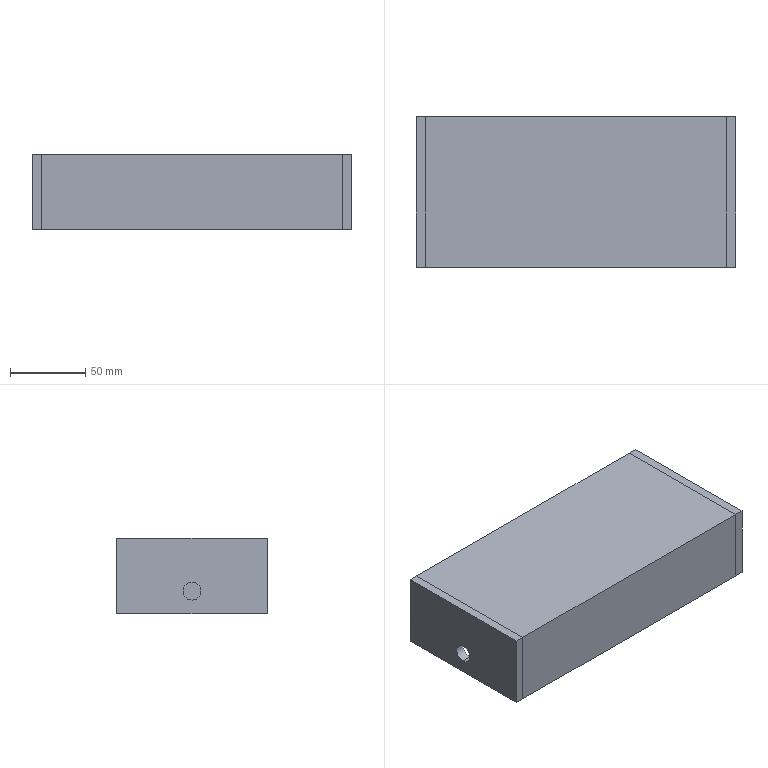Part | SolidWorks | features ICE 3, 3DProfileFeature 1, WeldMemberFeat 1, WeldmentFeature 1 | 3 solids | 28 faces | box 212 x 100 x 50 mm | volume 126521 mm3 | plane 26 | cylinder 2 | commonest cylinder face diameters 12 x2
STEP:
#1=CARTESIAN_POINT('',(0.,-50.,0.));
#2=VERTEX_POINT('',#1);
#3=CARTESIAN_POINT('',(0.,-50.,-50.));
#4=VERTEX_POINT('',#3);
#5=CARTESIAN_POINT('',(0.,-50.,0.));
#6=DIRECTION('',(0.,0.,-1.));
#7=VECTOR('',#6,1000.);
#8=LINE('',#5,#7);
#9=EDGE_CURVE('',#2,#4,#8,.T.);
#10=ORIENTED_EDGE('',*,*,#9,.T.);
#11=CARTESIAN_POINT('',(200.,-50.,-50.));
#12=VERTEX_POINT('',#11);
#13=CARTESIAN_POINT('',(200.,-50.,-50.));
#14=DIRECTION('',(-1.,0.,0.));
#15=VECTOR('',#14,1000.);
#16=LINE('',#13,#15);
#17=EDGE_CURVE('',#12,#4,#16,.T.);
#18=ORIENTED_EDGE('',*,*,#17,.F.);
#19=CARTESIAN_POINT('',(200.,-50.,0.));
#20=VERTEX_POINT('',#19);
#21=CARTESIAN_POINT('',(200.,-50.,0.));
#22=DIRECTION('',(0.,0.,-1.));
#23=VECTOR('',#22,1000.);
#24=LINE('',#21,#23);
#25=EDGE_CURVE('',#20,#12,#24,.T.);
#26=ORIENTED_EDGE('',*,*,#25,.F.);
#27=CARTESIAN_POINT('',(200.,-50.,0.));
#28=DIRECTION('',(-1.,0.,0.));
#29=VECTOR('',#28,1000.);
#30=LINE('',#27,#29);
#31=EDGE_CURVE('',#20,#2,#30,.T.);
#32=ORIENTED_EDGE('',*,*,#31,.T.);
#33=EDGE_LOOP('',(#10,#18,#26,#32));
#34=FACE_OUTER_BOUND('',#33,.T.);
#35=CARTESIAN_POINT('',(200.,-50.,0.));
#36=DIRECTION('',(0.,1.,0.));
#37=DIRECTION('',(0.,0.,1.));
#38=AXIS2_PLACEMENT_3D('',#35,#36,#37);
#39=PLANE('',#38);
#40=ADVANCED_FACE('',(#34),#39,.F.);
#41=CARTESIAN_POINT('',(0.,-35.,-50.));
#42=VERTEX_POINT('',#41);
#43=CARTESIAN_POINT('',(0.,-50.,-50.));
#44=DIRECTION('',(0.,1.,0.));
#45=VECTOR('',#44,1000.);
#46=LINE('',#43,#45);
#47=EDGE_CURVE('',#4,#42,#46,.T.);
#48=ORIENTED_EDGE('',*,*,#47,.T.);
#49=CARTESIAN_POINT('',(200.,-35.,-50.));
#50=VERTEX_POINT('',#49);
#51=CARTESIAN_POINT('',(200.,-35.,-50.));
#52=DIRECTION('',(-1.,0.,0.));
#53=VECTOR('',#52,1000.);
#54=LINE('',#51,#53);
#55=EDGE_CURVE('',#50,#42,#54,.T.);
#56=ORIENTED_EDGE('',*,*,#55,.F.);
#57=CARTESIAN_POINT('',(200.,-50.,-50.));
#58=DIRECTION('',(0.,1.,0.));
#59=VECTOR('',#58,1000.);
#60=LINE('',#57,#59);
#61=EDGE_CURVE('',#12,#50,#60,.T.);
#62=ORIENTED_EDGE('',*,*,#61,.F.);
#63=ORIENTED_EDGE('',*,*,#17,.T.);
#64=EDGE_LOOP('',(#48,#56,#62,#63));
#65=FACE_OUTER_BOUND('',#64,.T.);
#66=CARTESIAN_POINT('',(200.,-50.,-50.));
#67=DIRECTION('',(0.,0.,1.));
#68=DIRECTION('',(0.,-1.,0.));
#69=AXIS2_PLACEMENT_3D('',#66,#67,#68);
#70=PLANE('',#69);
#71=ADVANCED_FACE('',(#65),#70,.F.);
#72=CARTESIAN_POINT('',(0.,-35.,-48.5));
#73=VERTEX_POINT('',#72);
#74=CARTESIAN_POINT('',(0.,-35.,-48.5));
#75=DIRECTION('',(0.,0.,1.));
#76=VECTOR('',#75,1000.);
#77=LINE('',#74,#76);
#78=EDGE_CURVE('',#42,#73,#77,.T.);
#79=ORIENTED_EDGE('',*,*,#78,.T.);
#80=CARTESIAN_POINT('',(200.,-35.,-48.5));
#81=VERTEX_POINT('',#80);
#82=CARTESIAN_POINT('',(200.,-35.,-48.5));
#83=DIRECTION('',(-1.,0.,0.));
#84=VECTOR('',#83,1000.);
#85=LINE('',#82,#84);
#86=EDGE_CURVE('',#81,#73,#85,.T.);
#87=ORIENTED_EDGE('',*,*,#86,.F.);
#88=CARTESIAN_POINT('',(200.,-35.,-48.5));
#89=DIRECTION('',(0.,0.,1.));
#90=VECTOR('',#89,1000.);
#91=LINE('',#88,#90);
#92=EDGE_CURVE('',#50,#81,#91,.T.);
#93=ORIENTED_EDGE('',*,*,#92,.F.);
#94=ORIENTED_EDGE('',*,*,#55,.T.);
#95=EDGE_LOOP('',(#79,#87,#93,#94));
#96=FACE_OUTER_BOUND('',#95,.T.);
#97=CARTESIAN_POINT('',(200.,-35.,-48.5));
#98=DIRECTION('',(0.,-1.,0.));
#99=DIRECTION('',(0.,0.,-1.));
#100=AXIS2_PLACEMENT_3D('',#97,#98,#99);
#101=PLANE('',#100);
#102=ADVANCED_FACE('',(#96),#101,.F.);
#103=CARTESIAN_POINT('',(0.,-48.5,-48.5));
#104=VERTEX_POINT('',#103);
#105=CARTESIAN_POINT('',(0.,-48.5,-48.5));
#106=DIRECTION('',(0.,-1.,0.));
#107=VECTOR('',#106,1000.);
#108=LINE('',#105,#107);
#109=EDGE_CURVE('',#73,#104,#108,.T.);
#110=ORIENTED_EDGE('',*,*,#109,.T.);
#111=CARTESIAN_POINT('',(200.,-48.5,-48.5));
#112=VERTEX_POINT('',#111);
#113=CARTESIAN_POINT('',(200.,-48.5,-48.5));
#114=DIRECTION('',(-1.,0.,0.));
#115=VECTOR('',#114,1000.);
#116=LINE('',#113,#115);
#117=EDGE_CURVE('',#112,#104,#116,.T.);
#118=ORIENTED_EDGE('',*,*,#117,.F.);
#119=CARTESIAN_POINT('',(200.,-48.5,-48.5));
#120=DIRECTION('',(0.,-1.,0.));
#121=VECTOR('',#120,1000.);
#122=LINE('',#119,#121);
#123=EDGE_CURVE('',#81,#112,#122,.T.);
#124=ORIENTED_EDGE('',*,*,#123,.F.);
#125=ORIENTED_EDGE('',*,*,#86,.T.);
#126=EDGE_LOOP('',(#110,#118,#124,#125));
#127=FACE_OUTER_BOUND('',#126,.T.);
#128=CARTESIAN_POINT('',(200.,-48.5,-48.5));
#129=DIRECTION('',(0.,0.,-1.));
#130=DIRECTION('',(-1.,0.,0.));
#131=AXIS2_PLACEMENT_3D('',#128,#129,#130);
#132=PLANE('',#131);
#133=ADVANCED_FACE('',(#127),#132,.F.);
#134=CARTESIAN_POINT('',(0.,-48.5,-1.5));
#135=VERTEX_POINT('',#134);
#136=CARTESIAN_POINT('',(0.,-48.5,-1.5));
#137=DIRECTION('',(0.,0.,1.));
#138=VECTOR('',#137,1000.);
#139=LINE('',#136,#138);
#140=EDGE_CURVE('',#104,#135,#139,.T.);
#141=ORIENTED_EDGE('',*,*,#140,.T.);
#142=CARTESIAN_POINT('',(200.,-48.5,-1.5));
#143=VERTEX_POINT('',#142);
#144=CARTESIAN_POINT('',(200.,-48.5,-1.5));
#145=DIRECTION('',(-1.,0.,0.));
#146=VECTOR('',#145,1000.);
#147=LINE('',#144,#146);
#148=EDGE_CURVE('',#143,#135,#147,.T.);
#149=ORIENTED_EDGE('',*,*,#148,.F.);
#150=CARTESIAN_POINT('',(200.,-48.5,-1.5));
#151=DIRECTION('',(0.,0.,1.));
#152=VECTOR('',#151,1000.);
#153=LINE('',#150,#152);
#154=EDGE_CURVE('',#112,#143,#153,.T.);
#155=ORIENTED_EDGE('',*,*,#154,.F.);
#156=ORIENTED_EDGE('',*,*,#117,.T.);
#157=EDGE_LOOP('',(#141,#149,#155,#156));
#158=FACE_OUTER_BOUND('',#157,.T.);
#159=CARTESIAN_POINT('',(200.,-48.5,-1.5));
#160=DIRECTION('',(0.,-1.,0.));
#161=DIRECTION('',(0.,0.,-1.));
#162=AXIS2_PLACEMENT_3D('',#159,#160,#161);
#163=PLANE('',#162);
#164=ADVANCED_FACE('',(#158),#163,.F.);
#165=CARTESIAN_POINT('',(0.,48.5,-1.5));
#166=VERTEX_POINT('',#165);
#167=CARTESIAN_POINT('',(0.,48.5,-1.5));
#168=DIRECTION('',(0.,1.,0.));
#169=VECTOR('',#168,1000.);
#170=LINE('',#167,#169);
#171=EDGE_CURVE('',#135,#166,#170,.T.);
#172=ORIENTED_EDGE('',*,*,#171,.T.);
#173=CARTESIAN_POINT('',(200.,48.5,-1.5));
#174=VERTEX_POINT('',#173);
#175=CARTESIAN_POINT('',(200.,48.5,-1.5));
#176=DIRECTION('',(-1.,0.,0.));
#177=VECTOR('',#176,1000.);
#178=LINE('',#175,#177);
#179=EDGE_CURVE('',#174,#166,#178,.T.);
#180=ORIENTED_EDGE('',*,*,#179,.F.);
#181=CARTESIAN_POINT('',(200.,48.5,-1.5));
#182=DIRECTION('',(0.,1.,0.));
#183=VECTOR('',#182,1000.);
#184=LINE('',#181,#183);
#185=EDGE_CURVE('',#143,#174,#184,.T.);
#186=ORIENTED_EDGE('',*,*,#185,.F.);
#187=ORIENTED_EDGE('',*,*,#148,.T.);
#188=EDGE_LOOP('',(#172,#180,#186,#187));
#189=FACE_OUTER_BOUND('',#188,.T.);
#190=CARTESIAN_POINT('',(200.,48.5,-1.5));
#191=DIRECTION('',(0.,0.,1.));
#192=DIRECTION('',(0.,-1.,0.));
#193=AXIS2_PLACEMENT_3D('',#190,#191,#192);
#194=PLANE('',#193);
#195=ADVANCED_FACE('',(#189),#194,.F.);
#196=CARTESIAN_POINT('',(0.,48.5,-48.5));
#197=VERTEX_POINT('',#196);
#198=CARTESIAN_POINT('',(0.,48.5,-48.5));
#199=DIRECTION('',(0.,0.,-1.));
#200=VECTOR('',#199,1000.);
#201=LINE('',#198,#200);
#202=EDGE_CURVE('',#166,#197,#201,.T.);
#203=ORIENTED_EDGE('',*,*,#202,.T.);
#204=CARTESIAN_POINT('',(200.,48.5,-48.5));
#205=VERTEX_POINT('',#204);
#206=CARTESIAN_POINT('',(200.,48.5,-48.5));
#207=DIRECTION('',(-1.,0.,0.));
#208=VECTOR('',#207,1000.);
#209=LINE('',#206,#208);
#210=EDGE_CURVE('',#205,#197,#209,.T.);
#211=ORIENTED_EDGE('',*,*,#210,.F.);
#212=CARTESIAN_POINT('',(200.,48.5,-48.5));
#213=DIRECTION('',(0.,0.,-1.));
#214=VECTOR('',#213,1000.);
#215=LINE('',#212,#214);
#216=EDGE_CURVE('',#174,#205,#215,.T.);
#217=ORIENTED_EDGE('',*,*,#216,.F.);
#218=ORIENTED_EDGE('',*,*,#179,.T.);
#219=EDGE_LOOP('',(#203,#211,#217,#218));
#220=FACE_OUTER_BOUND('',#219,.T.);
#221=CARTESIAN_POINT('',(200.,48.5,-48.5));
#222=DIRECTION('',(0.,1.,0.));
#223=DIRECTION('',(0.,0.,1.));
#224=AXIS2_PLACEMENT_3D('',#221,#222,#223);
#225=PLANE('',#224);
#226=ADVANCED_FACE('',(#220),#225,.F.);
#227=CARTESIAN_POINT('',(0.,35.,-48.5));
#228=VERTEX_POINT('',#227);
#229=CARTESIAN_POINT('',(0.,35.,-48.5));
#230=DIRECTION('',(0.,-1.,0.));
#231=VECTOR('',#230,1000.);
#232=LINE('',#229,#231);
#233=EDGE_CURVE('',#197,#228,#232,.T.);
#234=ORIENTED_EDGE('',*,*,#233,.T.);
#235=CARTESIAN_POINT('',(200.,35.,-48.5));
#236=VERTEX_POINT('',#235);
#237=CARTESIAN_POINT('',(200.,35.,-48.5));
#238=DIRECTION('',(-1.,0.,0.));
#239=VECTOR('',#238,1000.);
#240=LINE('',#237,#239);
#241=EDGE_CURVE('',#236,#228,#240,.T.);
#242=ORIENTED_EDGE('',*,*,#241,.F.);
#243=CARTESIAN_POINT('',(200.,35.,-48.5));
#244=DIRECTION('',(0.,-1.,0.));
#245=VECTOR('',#244,1000.);
#246=LINE('',#243,#245);
#247=EDGE_CURVE('',#205,#236,#246,.T.);
#248=ORIENTED_EDGE('',*,*,#247,.F.);
#249=ORIENTED_EDGE('',*,*,#210,.T.);
#250=EDGE_LOOP('',(#234,#242,#248,#249));
#251=FACE_OUTER_BOUND('',#250,.T.);
#252=CARTESIAN_POINT('',(200.,35.,-48.5));
#253=DIRECTION('',(0.,0.,-1.));
#254=DIRECTION('',(-1.,0.,0.));
#255=AXIS2_PLACEMENT_3D('',#252,#253,#254);
#256=PLANE('',#255);
#257=ADVANCED_FACE('',(#251),#256,.F.);
#258=CARTESIAN_POINT('',(0.,35.,-50.));
#259=VERTEX_POINT('',#258);
#260=CARTESIAN_POINT('',(0.,35.,-50.));
#261=DIRECTION('',(0.,0.,-1.));
#262=VECTOR('',#261,1000.);
#263=LINE('',#260,#262);
#264=EDGE_CURVE('',#228,#259,#263,.T.);
#265=ORIENTED_EDGE('',*,*,#264,.T.);
#266=CARTESIAN_POINT('',(200.,35.,-50.));
#267=VERTEX_POINT('',#266);
#268=CARTESIAN_POINT('',(200.,35.,-50.));
#269=DIRECTION('',(-1.,0.,0.));
#270=VECTOR('',#269,1000.);
#271=LINE('',#268,#270);
#272=EDGE_CURVE('',#267,#259,#271,.T.);
#273=ORIENTED_EDGE('',*,*,#272,.F.);
#274=CARTESIAN_POINT('',(200.,35.,-50.));
#275=DIRECTION('',(0.,0.,-1.));
#276=VECTOR('',#275,1000.);
#277=LINE('',#274,#276);
#278=EDGE_CURVE('',#236,#267,#277,.T.);
#279=ORIENTED_EDGE('',*,*,#278,.F.);
#280=ORIENTED_EDGE('',*,*,#241,.T.);
#281=EDGE_LOOP('',(#265,#273,#279,#280));
#282=FACE_OUTER_BOUND('',#281,.T.);
#283=CARTESIAN_POINT('',(200.,35.,-50.));
#284=DIRECTION('',(0.,1.,0.));
#285=DIRECTION('',(0.,0.,1.));
#286=AXIS2_PLACEMENT_3D('',#283,#284,#285);
#287=PLANE('',#286);
#288=ADVANCED_FACE('',(#282),#287,.F.);
#289=CARTESIAN_POINT('',(0.,50.,-50.));
#290=VERTEX_POINT('',#289);
#291=CARTESIAN_POINT('',(0.,50.,-50.));
#292=DIRECTION('',(0.,1.,0.));
#293=VECTOR('',#292,1000.);
#294=LINE('',#291,#293);
#295=EDGE_CURVE('',#259,#290,#294,.T.);
#296=ORIENTED_EDGE('',*,*,#295,.T.);
#297=CARTESIAN_POINT('',(200.,50.,-50.));
#298=VERTEX_POINT('',#297);
#299=CARTESIAN_POINT('',(200.,50.,-50.));
#300=DIRECTION('',(-1.,0.,0.));
#301=VECTOR('',#300,1000.);
#302=LINE('',#299,#301);
#303=EDGE_CURVE('',#298,#290,#302,.T.);
#304=ORIENTED_EDGE('',*,*,#303,.F.);
#305=CARTESIAN_POINT('',(200.,50.,-50.));
#306=DIRECTION('',(0.,1.,0.));
#307=VECTOR('',#306,1000.);
#308=LINE('',#305,#307);
#309=EDGE_CURVE('',#267,#298,#308,.T.);
#310=ORIENTED_EDGE('',*,*,#309,.F.);
#311=ORIENTED_EDGE('',*,*,#272,.T.);
#312=EDGE_LOOP('',(#296,#304,#310,#311));
#313=FACE_OUTER_BOUND('',#312,.T.);
#314=CARTESIAN_POINT('',(200.,50.,-50.));
#315=DIRECTION('',(0.,0.,1.));
#316=DIRECTION('',(0.,-1.,0.));
#317=AXIS2_PLACEMENT_3D('',#314,#315,#316);
#318=PLANE('',#317);
#319=ADVANCED_FACE('',(#313),#318,.F.);
#320=CARTESIAN_POINT('',(0.,50.,0.));
#321=VERTEX_POINT('',#320);
#322=CARTESIAN_POINT('',(0.,50.,0.));
#323=DIRECTION('',(0.,0.,1.));
#324=VECTOR('',#323,1000.);
#325=LINE('',#322,#324);
#326=EDGE_CURVE('',#290,#321,#325,.T.);
#327=ORIENTED_EDGE('',*,*,#326,.T.);
#328=CARTESIAN_POINT('',(200.,50.,0.));
#329=VERTEX_POINT('',#328);
#330=CARTESIAN_POINT('',(200.,50.,0.));
#331=DIRECTION('',(-1.,0.,0.));
#332=VECTOR('',#331,1000.);
#333=LINE('',#330,#332);
#334=EDGE_CURVE('',#329,#321,#333,.T.);
#335=ORIENTED_EDGE('',*,*,#334,.F.);
#336=CARTESIAN_POINT('',(200.,50.,0.));
#337=DIRECTION('',(0.,0.,1.));
#338=VECTOR('',#337,1000.);
#339=LINE('',#336,#338);
#340=EDGE_CURVE('',#298,#329,#339,.T.);
#341=ORIENTED_EDGE('',*,*,#340,.F.);
#342=ORIENTED_EDGE('',*,*,#303,.T.);
#343=EDGE_LOOP('',(#327,#335,#341,#342));
#344=FACE_OUTER_BOUND('',#343,.T.);
#345=CARTESIAN_POINT('',(200.,50.,0.));
#346=DIRECTION('',(0.,-1.,0.));
#347=DIRECTION('',(0.,0.,-1.));
#348=AXIS2_PLACEMENT_3D('',#345,#346,#347);
#349=PLANE('',#348);
#350=ADVANCED_FACE('',(#344),#349,.F.);
#351=CARTESIAN_POINT('',(0.,-50.,0.));
#352=DIRECTION('',(0.,-1.,0.));
#353=VECTOR('',#352,1000.);
#354=LINE('',#351,#353);
#355=EDGE_CURVE('',#321,#2,#354,.T.);
#356=ORIENTED_EDGE('',*,*,#355,.T.);
#357=ORIENTED_EDGE('',*,*,#31,.F.);
#358=CARTESIAN_POINT('',(200.,-50.,0.));
#359=DIRECTION('',(0.,-1.,0.));
#360=VECTOR('',#359,1000.);
#361=LINE('',#358,#360);
#362=EDGE_CURVE('',#329,#20,#361,.T.);
#363=ORIENTED_EDGE('',*,*,#362,.F.);
#364=ORIENTED_EDGE('',*,*,#334,.T.);
#365=EDGE_LOOP('',(#356,#357,#363,#364));
#366=FACE_OUTER_BOUND('',#365,.T.);
#367=CARTESIAN_POINT('',(200.,-50.,0.));
#368=DIRECTION('',(0.,0.,-1.));
#369=DIRECTION('',(-1.,0.,0.));
#370=AXIS2_PLACEMENT_3D('',#367,#368,#369);
#371=PLANE('',#370);
#372=ADVANCED_FACE('',(#366),#371,.F.);
#373=ORIENTED_EDGE('',*,*,#25,.T.);
#374=ORIENTED_EDGE('',*,*,#61,.T.);
#375=ORIENTED_EDGE('',*,*,#92,.T.);
#376=ORIENTED_EDGE('',*,*,#123,.T.);
#377=ORIENTED_EDGE('',*,*,#154,.T.);
#378=ORIENTED_EDGE('',*,*,#185,.T.);
#379=ORIENTED_EDGE('',*,*,#216,.T.);
#380=ORIENTED_EDGE('',*,*,#247,.T.);
#381=ORIENTED_EDGE('',*,*,#278,.T.);
#382=ORIENTED_EDGE('',*,*,#309,.T.);
#383=ORIENTED_EDGE('',*,*,#340,.T.);
#384=ORIENTED_EDGE('',*,*,#362,.T.);
#385=EDGE_LOOP('',(#373,#374,#375,#376,#377,#378,#379,#380,#381,#382,#383,#384));
#386=FACE_OUTER_BOUND('',#385,.T.);
#387=CARTESIAN_POINT('',(200.,0.,0.));
#388=DIRECTION('',(1.,0.,0.));
#389=DIRECTION('',(0.,0.,-1.));
#390=AXIS2_PLACEMENT_3D('',#387,#388,#389);
#391=PLANE('',#390);
#392=ADVANCED_FACE('',(#386),#391,.T.);
#393=ORIENTED_EDGE('',*,*,#9,.F.);
#394=ORIENTED_EDGE('',*,*,#355,.F.);
#395=ORIENTED_EDGE('',*,*,#326,.F.);
#396=ORIENTED_EDGE('',*,*,#295,.F.);
#397=ORIENTED_EDGE('',*,*,#264,.F.);
#398=ORIENTED_EDGE('',*,*,#233,.F.);
#399=ORIENTED_EDGE('',*,*,#202,.F.);
#400=ORIENTED_EDGE('',*,*,#171,.F.);
#401=ORIENTED_EDGE('',*,*,#140,.F.);
#402=ORIENTED_EDGE('',*,*,#109,.F.);
#403=ORIENTED_EDGE('',*,*,#78,.F.);
#404=ORIENTED_EDGE('',*,*,#47,.F.);
#405=EDGE_LOOP('',(#393,#394,#395,#396,#397,#398,#399,#400,#401,#402,#403,#404));
#406=FACE_OUTER_BOUND('',#405,.T.);
#407=CARTESIAN_POINT('',(0.,0.,0.));
#408=DIRECTION('',(1.,0.,0.));
#409=DIRECTION('',(0.,0.,-1.));
#410=AXIS2_PLACEMENT_3D('',#407,#408,#409);
#411=PLANE('',#410);
#412=ADVANCED_FACE('',(#406),#411,.F.);
#413=CLOSED_SHELL('',(#40,#71,#102,#133,#164,#195,#226,#257,#288,#319,#350,#372,#392,#412));
#414=MANIFOLD_SOLID_BREP('',#413);
#415=CARTESIAN_POINT('',(200.,50.,0.));
#416=VERTEX_POINT('',#415);
#417=CARTESIAN_POINT('',(200.,-50.,0.));
#418=VERTEX_POINT('',#417);
#419=CARTESIAN_POINT('',(200.,50.,0.));
#420=DIRECTION('',(0.,-1.,0.));
#421=VECTOR('',#420,1000.);
#422=LINE('',#419,#421);
#423=EDGE_CURVE('',#416,#418,#422,.T.);
#424=ORIENTED_EDGE('',*,*,#423,.T.);
#425=CARTESIAN_POINT('',(206.,-50.,0.));
#426=VERTEX_POINT('',#425);
#427=CARTESIAN_POINT('',(206.,-50.,0.));
#428=DIRECTION('',(-1.,0.,0.));
#429=VECTOR('',#428,1000.);
#430=LINE('',#427,#429);
#431=EDGE_CURVE('',#426,#418,#430,.T.);
#432=ORIENTED_EDGE('',*,*,#431,.F.);
#433=CARTESIAN_POINT('',(206.,50.,0.));
#434=VERTEX_POINT('',#433);
#435=CARTESIAN_POINT('',(206.,50.,0.));
#436=DIRECTION('',(0.,-1.,0.));
#437=VECTOR('',#436,1000.);
#438=LINE('',#435,#437);
#439=EDGE_CURVE('',#434,#426,#438,.T.);
#440=ORIENTED_EDGE('',*,*,#439,.F.);
#441=CARTESIAN_POINT('',(206.,50.,0.));
#442=DIRECTION('',(-1.,0.,0.));
#443=VECTOR('',#442,1000.);
#444=LINE('',#441,#443);
#445=EDGE_CURVE('',#434,#416,#444,.T.);
#446=ORIENTED_EDGE('',*,*,#445,.T.);
#447=EDGE_LOOP('',(#424,#432,#440,#446));
#448=FACE_OUTER_BOUND('',#447,.T.);
#449=CARTESIAN_POINT('',(206.,50.,0.));
#450=DIRECTION('',(0.,0.,-1.));
#451=DIRECTION('',(0.,1.,0.));
#452=AXIS2_PLACEMENT_3D('',#449,#450,#451);
#453=PLANE('',#452);
#454=ADVANCED_FACE('',(#448),#453,.F.);
#455=CARTESIAN_POINT('',(200.,-50.,-50.));
#456=VERTEX_POINT('',#455);
#457=CARTESIAN_POINT('',(200.,-50.,0.));
#458=DIRECTION('',(0.,0.,-1.));
#459=VECTOR('',#458,1000.);
#460=LINE('',#457,#459);
#461=EDGE_CURVE('',#418,#456,#460,.T.);
#462=ORIENTED_EDGE('',*,*,#461,.T.);
#463=CARTESIAN_POINT('',(206.,-50.,-50.));
#464=VERTEX_POINT('',#463);
#465=CARTESIAN_POINT('',(206.,-50.,-50.));
#466=DIRECTION('',(-1.,0.,0.));
#467=VECTOR('',#466,1000.);
#468=LINE('',#465,#467);
#469=EDGE_CURVE('',#464,#456,#468,.T.);
#470=ORIENTED_EDGE('',*,*,#469,.F.);
#471=CARTESIAN_POINT('',(206.,-50.,0.));
#472=DIRECTION('',(0.,0.,-1.));
#473=VECTOR('',#472,1000.);
#474=LINE('',#471,#473);
#475=EDGE_CURVE('',#426,#464,#474,.T.);
#476=ORIENTED_EDGE('',*,*,#475,.F.);
#477=ORIENTED_EDGE('',*,*,#431,.T.);
#478=EDGE_LOOP('',(#462,#470,#476,#477));
#479=FACE_OUTER_BOUND('',#478,.T.);
#480=CARTESIAN_POINT('',(206.,-50.,0.));
#481=DIRECTION('',(0.,1.,0.));
#482=DIRECTION('',(0.,0.,1.));
#483=AXIS2_PLACEMENT_3D('',#480,#481,#482);
#484=PLANE('',#483);
#485=ADVANCED_FACE('',(#479),#484,.F.);
#486=CARTESIAN_POINT('',(200.,50.,-50.));
#487=VERTEX_POINT('',#486);
#488=CARTESIAN_POINT('',(200.,50.,-50.));
#489=DIRECTION('',(0.,1.,0.));
#490=VECTOR('',#489,1000.);
#491=LINE('',#488,#490);
#492=EDGE_CURVE('',#456,#487,#491,.T.);
#493=ORIENTED_EDGE('',*,*,#492,.T.);
#494=CARTESIAN_POINT('',(206.,50.,-50.));
#495=VERTEX_POINT('',#494);
#496=CARTESIAN_POINT('',(206.,50.,-50.));
#497=DIRECTION('',(-1.,0.,0.));
#498=VECTOR('',#497,1000.);
#499=LINE('',#496,#498);
#500=EDGE_CURVE('',#495,#487,#499,.T.);
#501=ORIENTED_EDGE('',*,*,#500,.F.);
#502=CARTESIAN_POINT('',(206.,50.,-50.));
#503=DIRECTION('',(0.,1.,0.));
#504=VECTOR('',#503,1000.);
#505=LINE('',#502,#504);
#506=EDGE_CURVE('',#464,#495,#505,.T.);
#507=ORIENTED_EDGE('',*,*,#506,.F.);
#508=ORIENTED_EDGE('',*,*,#469,.T.);
#509=EDGE_LOOP('',(#493,#501,#507,#508));
#510=FACE_OUTER_BOUND('',#509,.T.);
#511=CARTESIAN_POINT('',(206.,50.,-50.));
#512=DIRECTION('',(0.,0.,1.));
#513=DIRECTION('',(0.,-1.,0.));
#514=AXIS2_PLACEMENT_3D('',#511,#512,#513);
#515=PLANE('',#514);
#516=ADVANCED_FACE('',(#510),#515,.F.);
#517=CARTESIAN_POINT('',(200.,50.,0.));
#518=DIRECTION('',(0.,0.,1.));
#519=VECTOR('',#518,1000.);
#520=LINE('',#517,#519);
#521=EDGE_CURVE('',#487,#416,#520,.T.);
#522=ORIENTED_EDGE('',*,*,#521,.T.);
#523=ORIENTED_EDGE('',*,*,#445,.F.);
#524=CARTESIAN_POINT('',(206.,50.,0.));
#525=DIRECTION('',(0.,0.,1.));
#526=VECTOR('',#525,1000.);
#527=LINE('',#524,#526);
#528=EDGE_CURVE('',#495,#434,#527,.T.);
#529=ORIENTED_EDGE('',*,*,#528,.F.);
#530=ORIENTED_EDGE('',*,*,#500,.T.);
#531=EDGE_LOOP('',(#522,#523,#529,#530));
#532=FACE_OUTER_BOUND('',#531,.T.);
#533=CARTESIAN_POINT('',(206.,50.,0.));
#534=DIRECTION('',(0.,-1.,0.));
#535=DIRECTION('',(0.,0.,-1.));
#536=AXIS2_PLACEMENT_3D('',#533,#534,#535);
#537=PLANE('',#536);
#538=ADVANCED_FACE('',(#532),#537,.F.);
#539=ORIENTED_EDGE('',*,*,#439,.T.);
#540=ORIENTED_EDGE('',*,*,#475,.T.);
#541=ORIENTED_EDGE('',*,*,#506,.T.);
#542=ORIENTED_EDGE('',*,*,#528,.T.);
#543=EDGE_LOOP('',(#539,#540,#541,#542));
#544=FACE_OUTER_BOUND('',#543,.T.);
#545=CARTESIAN_POINT('',(206.,0.,0.));
#546=DIRECTION('',(1.,0.,0.));
#547=DIRECTION('',(0.,0.,-1.));
#548=AXIS2_PLACEMENT_3D('',#545,#546,#547);
#549=PLANE('',#548);
#550=ADVANCED_FACE('',(#544),#549,.T.);
#551=ORIENTED_EDGE('',*,*,#423,.F.);
#552=ORIENTED_EDGE('',*,*,#521,.F.);
#553=ORIENTED_EDGE('',*,*,#492,.F.);
#554=ORIENTED_EDGE('',*,*,#461,.F.);
#555=EDGE_LOOP('',(#551,#552,#553,#554));
#556=FACE_OUTER_BOUND('',#555,.T.);
#557=CARTESIAN_POINT('',(200.,0.,0.));
#558=DIRECTION('',(1.,0.,0.));
#559=DIRECTION('',(0.,0.,-1.));
#560=AXIS2_PLACEMENT_3D('',#557,#558,#559);
#561=PLANE('',#560);
#562=ADVANCED_FACE('',(#556),#561,.F.);
#563=CLOSED_SHELL('',(#454,#485,#516,#538,#550,#562));
#564=MANIFOLD_SOLID_BREP('',#563);
#565=CARTESIAN_POINT('',(0.,0.,-41.));
#566=VERTEX_POINT('',#565);
#567=CARTESIAN_POINT('',(0.,0.,-29.));
#568=VERTEX_POINT('',#567);
#569=CARTESIAN_POINT('',(0.,0.,-35.));
#570=DIRECTION('',(-1.,0.,0.));
#571=DIRECTION('',(0.,0.,1.));
#572=AXIS2_PLACEMENT_3D('',#569,#570,#571);
#573=CIRCLE('',#572,6.);
#574=EDGE_CURVE('',#566,#568,#573,.T.);
#575=ORIENTED_EDGE('',*,*,#574,.F.);
#576=CARTESIAN_POINT('',(-6.,0.,-41.));
#577=VERTEX_POINT('',#576);
#578=CARTESIAN_POINT('',(8.,0.,-41.));
#579=DIRECTION('',(-1.,0.,0.));
#580=VECTOR('',#579,1000.);
#581=LINE('',#578,#580);
#582=EDGE_CURVE('',#566,#577,#581,.T.);
#583=ORIENTED_EDGE('',*,*,#582,.T.);
#584=CARTESIAN_POINT('',(-6.,0.,-29.));
#585=VERTEX_POINT('',#584);
#586=CARTESIAN_POINT('',(-6.,0.,-35.));
#587=DIRECTION('',(-1.,0.,0.));
#588=DIRECTION('',(0.,0.,1.));
#589=AXIS2_PLACEMENT_3D('',#586,#587,#588);
#590=CIRCLE('',#589,6.);
#591=EDGE_CURVE('',#577,#585,#590,.T.);
#592=ORIENTED_EDGE('',*,*,#591,.T.);
#593=CARTESIAN_POINT('',(8.,0.,-29.));
#594=DIRECTION('',(-1.,0.,0.));
#595=VECTOR('',#594,1000.);
#596=LINE('',#593,#595);
#597=EDGE_CURVE('',#568,#585,#596,.T.);
#598=ORIENTED_EDGE('',*,*,#597,.F.);
#599=EDGE_LOOP('',(#575,#583,#592,#598));
#600=FACE_OUTER_BOUND('',#599,.T.);
#601=CARTESIAN_POINT('',(8.,0.,-35.));
#602=DIRECTION('',(-1.,0.,0.));
#603=DIRECTION('',(0.,0.,1.));
#604=AXIS2_PLACEMENT_3D('',#601,#602,#603);
#605=CYLINDRICAL_SURFACE('',#604,6.);
#606=ADVANCED_FACE('',(#600),#605,.F.);
#607=CARTESIAN_POINT('',(0.,50.,-50.));
#608=VERTEX_POINT('',#607);
#609=CARTESIAN_POINT('',(0.,-50.,-50.));
#610=VERTEX_POINT('',#609);
#611=CARTESIAN_POINT('',(0.,50.,-50.));
#612=DIRECTION('',(0.,-1.,0.));
#613=VECTOR('',#612,1000.);
#614=LINE('',#611,#613);
#615=EDGE_CURVE('',#608,#610,#614,.T.);
#616=ORIENTED_EDGE('',*,*,#615,.T.);
#617=CARTESIAN_POINT('',(-6.,-50.,-50.));
#618=VERTEX_POINT('',#617);
#619=CARTESIAN_POINT('',(-6.,-50.,-50.));
#620=DIRECTION('',(1.,0.,0.));
#621=VECTOR('',#620,1000.);
#622=LINE('',#619,#621);
#623=EDGE_CURVE('',#618,#610,#622,.T.);
#624=ORIENTED_EDGE('',*,*,#623,.F.);
#625=CARTESIAN_POINT('',(-6.,50.,-50.));
#626=VERTEX_POINT('',#625);
#627=CARTESIAN_POINT('',(-6.,50.,-50.));
#628=DIRECTION('',(0.,-1.,0.));
#629=VECTOR('',#628,1000.);
#630=LINE('',#627,#629);
#631=EDGE_CURVE('',#626,#618,#630,.T.);
#632=ORIENTED_EDGE('',*,*,#631,.F.);
#633=CARTESIAN_POINT('',(-6.,50.,-50.));
#634=DIRECTION('',(1.,0.,0.));
#635=VECTOR('',#634,1000.);
#636=LINE('',#633,#635);
#637=EDGE_CURVE('',#626,#608,#636,.T.);
#638=ORIENTED_EDGE('',*,*,#637,.T.);
#639=EDGE_LOOP('',(#616,#624,#632,#638));
#640=FACE_OUTER_BOUND('',#639,.T.);
#641=CARTESIAN_POINT('',(-6.,50.,-50.));
#642=DIRECTION('',(0.,0.,1.));
#643=DIRECTION('',(0.,-1.,0.));
#644=AXIS2_PLACEMENT_3D('',#641,#642,#643);
#645=PLANE('',#644);
#646=ADVANCED_FACE('',(#640),#645,.F.);
#647=CARTESIAN_POINT('',(0.,-50.,0.));
#648=VERTEX_POINT('',#647);
#649=CARTESIAN_POINT('',(0.,-50.,-50.));
#650=DIRECTION('',(0.,0.,1.));
#651=VECTOR('',#650,1000.);
#652=LINE('',#649,#651);
#653=EDGE_CURVE('',#610,#648,#652,.T.);
#654=ORIENTED_EDGE('',*,*,#653,.T.);
#655=CARTESIAN_POINT('',(-6.,-50.,0.));
#656=VERTEX_POINT('',#655);
#657=CARTESIAN_POINT('',(-6.,-50.,0.));
#658=DIRECTION('',(1.,0.,0.));
#659=VECTOR('',#658,1000.);
#660=LINE('',#657,#659);
#661=EDGE_CURVE('',#656,#648,#660,.T.);
#662=ORIENTED_EDGE('',*,*,#661,.F.);
#663=CARTESIAN_POINT('',(-6.,-50.,-50.));
#664=DIRECTION('',(0.,0.,1.));
#665=VECTOR('',#664,1000.);
#666=LINE('',#663,#665);
#667=EDGE_CURVE('',#618,#656,#666,.T.);
#668=ORIENTED_EDGE('',*,*,#667,.F.);
#669=ORIENTED_EDGE('',*,*,#623,.T.);
#670=EDGE_LOOP('',(#654,#662,#668,#669));
#671=FACE_OUTER_BOUND('',#670,.T.);
#672=CARTESIAN_POINT('',(-6.,-50.,-50.));
#673=DIRECTION('',(0.,1.,0.));
#674=DIRECTION('',(0.,0.,1.));
#675=AXIS2_PLACEMENT_3D('',#672,#673,#674);
#676=PLANE('',#675);
#677=ADVANCED_FACE('',(#671),#676,.F.);
#678=CARTESIAN_POINT('',(0.,50.,0.));
#679=VERTEX_POINT('',#678);
#680=CARTESIAN_POINT('',(0.,50.,0.));
#681=DIRECTION('',(0.,1.,0.));
#682=VECTOR('',#681,1000.);
#683=LINE('',#680,#682);
#684=EDGE_CURVE('',#648,#679,#683,.T.);
#685=ORIENTED_EDGE('',*,*,#684,.T.);
#686=CARTESIAN_POINT('',(-6.,50.,0.));
#687=VERTEX_POINT('',#686);
#688=CARTESIAN_POINT('',(-6.,50.,0.));
#689=DIRECTION('',(1.,0.,0.));
#690=VECTOR('',#689,1000.);
#691=LINE('',#688,#690);
#692=EDGE_CURVE('',#687,#679,#691,.T.);
#693=ORIENTED_EDGE('',*,*,#692,.F.);
#694=CARTESIAN_POINT('',(-6.,50.,0.));
#695=DIRECTION('',(0.,1.,0.));
#696=VECTOR('',#695,1000.);
#697=LINE('',#694,#696);
#698=EDGE_CURVE('',#656,#687,#697,.T.);
#699=ORIENTED_EDGE('',*,*,#698,.F.);
#700=ORIENTED_EDGE('',*,*,#661,.T.);
#701=EDGE_LOOP('',(#685,#693,#699,#700));
#702=FACE_OUTER_BOUND('',#701,.T.);
#703=CARTESIAN_POINT('',(-6.,50.,0.));
#704=DIRECTION('',(0.,0.,-1.));
#705=DIRECTION('',(0.,1.,0.));
#706=AXIS2_PLACEMENT_3D('',#703,#704,#705);
#707=PLANE('',#706);
#708=ADVANCED_FACE('',(#702),#707,.F.);
#709=CARTESIAN_POINT('',(0.,50.,-50.));
#710=DIRECTION('',(0.,0.,-1.));
#711=VECTOR('',#710,1000.);
#712=LINE('',#709,#711);
#713=EDGE_CURVE('',#679,#608,#712,.T.);
#714=ORIENTED_EDGE('',*,*,#713,.T.);
#715=ORIENTED_EDGE('',*,*,#637,.F.);
#716=CARTESIAN_POINT('',(-6.,50.,-50.));
#717=DIRECTION('',(0.,0.,-1.));
#718=VECTOR('',#717,1000.);
#719=LINE('',#716,#718);
#720=EDGE_CURVE('',#687,#626,#719,.T.);
#721=ORIENTED_EDGE('',*,*,#720,.F.);
#722=ORIENTED_EDGE('',*,*,#692,.T.);
#723=EDGE_LOOP('',(#714,#715,#721,#722));
#724=FACE_OUTER_BOUND('',#723,.T.);
#725=CARTESIAN_POINT('',(-6.,50.,-50.));
#726=DIRECTION('',(0.,-1.,0.));
#727=DIRECTION('',(0.,0.,-1.));
#728=AXIS2_PLACEMENT_3D('',#725,#726,#727);
#729=PLANE('',#728);
#730=ADVANCED_FACE('',(#724),#729,.F.);
#731=CARTESIAN_POINT('',(-6.,0.,-35.));
#732=DIRECTION('',(-1.,0.,0.));
#733=DIRECTION('',(0.,0.,1.));
#734=AXIS2_PLACEMENT_3D('',#731,#732,#733);
#735=CIRCLE('',#734,6.);
#736=EDGE_CURVE('',#585,#577,#735,.T.);
#737=ORIENTED_EDGE('',*,*,#736,.F.);
#738=ORIENTED_EDGE('',*,*,#591,.F.);
#739=EDGE_LOOP('',(#737,#738));
#740=FACE_BOUND('',#739,.T.);
#741=ORIENTED_EDGE('',*,*,#631,.T.);
#742=ORIENTED_EDGE('',*,*,#667,.T.);
#743=ORIENTED_EDGE('',*,*,#698,.T.);
#744=ORIENTED_EDGE('',*,*,#720,.T.);
#745=EDGE_LOOP('',(#741,#742,#743,#744));
#746=FACE_OUTER_BOUND('',#745,.T.);
#747=CARTESIAN_POINT('',(-6.,0.,0.));
#748=DIRECTION('',(-1.,0.,0.));
#749=DIRECTION('',(0.,0.,1.));
#750=AXIS2_PLACEMENT_3D('',#747,#748,#749);
#751=PLANE('',#750);
#752=ADVANCED_FACE('',(#740,#746),#751,.T.);
#753=CARTESIAN_POINT('',(0.,0.,-35.));
#754=DIRECTION('',(-1.,0.,0.));
#755=DIRECTION('',(0.,0.,1.));
#756=AXIS2_PLACEMENT_3D('',#753,#754,#755);
#757=CIRCLE('',#756,6.);
#758=EDGE_CURVE('',#568,#566,#757,.T.);
#759=ORIENTED_EDGE('',*,*,#758,.T.);
#760=ORIENTED_EDGE('',*,*,#574,.T.);
#761=EDGE_LOOP('',(#759,#760));
#762=FACE_BOUND('',#761,.T.);
#763=ORIENTED_EDGE('',*,*,#615,.F.);
#764=ORIENTED_EDGE('',*,*,#713,.F.);
#765=ORIENTED_EDGE('',*,*,#684,.F.);
#766=ORIENTED_EDGE('',*,*,#653,.F.);
#767=EDGE_LOOP('',(#763,#764,#765,#766));
#768=FACE_OUTER_BOUND('',#767,.T.);
#769=CARTESIAN_POINT('',(0.,0.,0.));
#770=DIRECTION('',(-1.,0.,0.));
#771=DIRECTION('',(0.,0.,1.));
#772=AXIS2_PLACEMENT_3D('',#769,#770,#771);
#773=PLANE('',#772);
#774=ADVANCED_FACE('',(#762,#768),#773,.F.);
#775=ORIENTED_EDGE('',*,*,#582,.F.);
#776=ORIENTED_EDGE('',*,*,#758,.F.);
#777=ORIENTED_EDGE('',*,*,#597,.T.);
#778=ORIENTED_EDGE('',*,*,#736,.T.);
#779=EDGE_LOOP('',(#775,#776,#777,#778));
#780=FACE_OUTER_BOUND('',#779,.T.);
#781=CARTESIAN_POINT('',(8.,0.,-35.));
#782=DIRECTION('',(-1.,0.,0.));
#783=DIRECTION('',(0.,0.,1.));
#784=AXIS2_PLACEMENT_3D('',#781,#782,#783);
#785=CYLINDRICAL_SURFACE('',#784,6.);
#786=ADVANCED_FACE('',(#780),#785,.F.);
#787=CLOSED_SHELL('',(#606,#646,#677,#708,#730,#752,#774,#786));
#788=MANIFOLD_SOLID_BREP('',#787);
#789=CARTESIAN_POINT('',(0.,0.,0.));
#790=DIRECTION('',(0.,0.,1.));
#791=DIRECTION('',(1.,0.,0.));
#792=AXIS2_PLACEMENT_3D('',#789,#790,#791);
#793=(LENGTH_UNIT()NAMED_UNIT(*)SI_UNIT(.MILLI.,.METRE.));
#794=UNCERTAINTY_MEASURE_WITH_UNIT(LENGTH_MEASURE(0.00001),#793,'','');
#795=(NAMED_UNIT(*)PLANE_ANGLE_UNIT()SI_UNIT($,.RADIAN.));
#796=(NAMED_UNIT(*)SI_UNIT($,.STERADIAN.)SOLID_ANGLE_UNIT());
#797=(GEOMETRIC_REPRESENTATION_CONTEXT(3)GLOBAL_UNCERTAINTY_ASSIGNED_CONTEXT((#794))GLOBAL_UNIT_ASSIGNED_CONTEXT((#793,#795,#796))REPRESENTATION_CONTEXT('',''));
#798=ADVANCED_BREP_SHAPE_REPRESENTATION('',(#414,#564,#788,#792),#797);